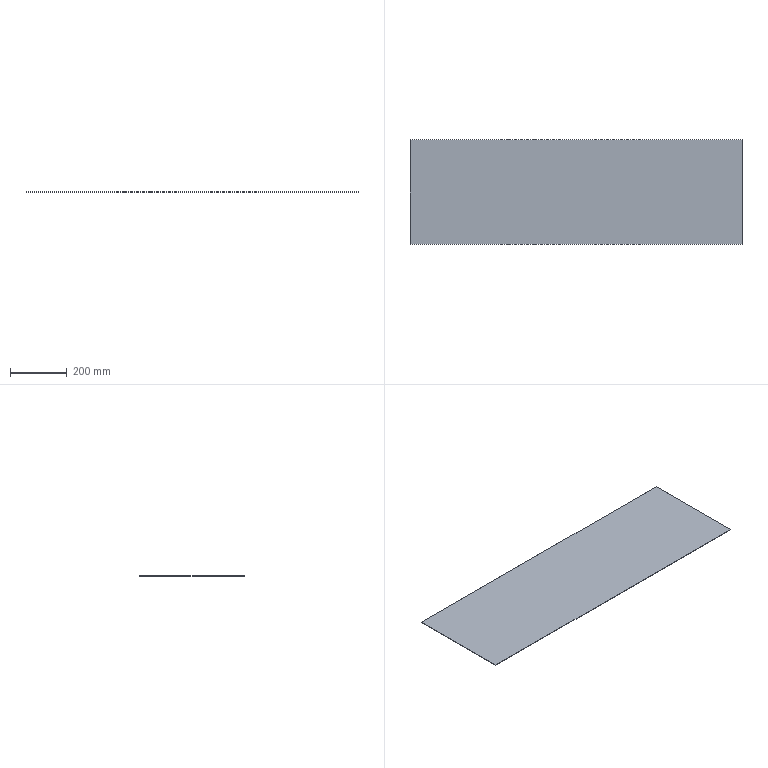Part | STEP file | JZBM | 1 solid | 6 faces | box 1170 x 370 x 1.5 mm | volume 649350 mm3 | plane 6
STEP:
#1=CARTESIAN_POINT('',(0.,0.,0.));
#2=DIRECTION('',(0.,0.,1.));
#3=DIRECTION('',(1.,0.,0.));
#4=AXIS2_PLACEMENT_3D('',#1,#2,#3);
#5=CARTESIAN_POINT('',(-585.,185.,0.));
#6=VERTEX_POINT('',#5);
#7=CARTESIAN_POINT('',(-585.,-185.,0.));
#8=VERTEX_POINT('',#7);
#9=CARTESIAN_POINT('',(-585.,185.,0.));
#10=DIRECTION('',(0.,-1.,0.));
#11=VECTOR('',#10,1.);
#12=LINE('',#9,#11);
#13=CARTESIAN_POINT('',(-585.,185.,1.5));
#14=DIRECTION('',(1.,0.,0.));
#15=DIRECTION('',(0.,0.,-1.));
#16=AXIS2_PLACEMENT_3D('',#13,#14,#15);
#17=PLANE('',#16);
#18=CARTESIAN_POINT('',(1.5,0.));
#19=DIRECTION('',(0.,-1.));
#20=VECTOR('',#19,1.);
#21=LINE('',#18,#20);
#22=(GEOMETRIC_REPRESENTATION_CONTEXT(2)PARAMETRIC_REPRESENTATION_CONTEXT()REPRESENTATION_CONTEXT('',''));
#23=DEFINITIONAL_REPRESENTATION('',(#21),#22);
#24=PCURVE('',#17,#23);
#25=CARTESIAN_POINT('',(-585.,-185.,0.));
#26=DIRECTION('',(0.,0.,1.));
#27=DIRECTION('',(1.,0.,0.));
#28=AXIS2_PLACEMENT_3D('',#25,#26,#27);
#29=PLANE('',#28);
#30=CARTESIAN_POINT('',(0.,370.));
#31=DIRECTION('',(0.,-1.));
#32=VECTOR('',#31,1.);
#33=LINE('',#30,#32);
#34=(GEOMETRIC_REPRESENTATION_CONTEXT(2)PARAMETRIC_REPRESENTATION_CONTEXT()REPRESENTATION_CONTEXT('',''));
#35=DEFINITIONAL_REPRESENTATION('',(#33),#34);
#36=PCURVE('',#29,#35);
#37=SURFACE_CURVE('',#12,(#24,#36),.PCURVE_S1.);
#38=EDGE_CURVE('',#6,#8,#37,.T.);
#39=ORIENTED_EDGE('',*,*,#38,.T.);
#40=CARTESIAN_POINT('',(-585.,-185.,1.5));
#41=VERTEX_POINT('',#40);
#42=CARTESIAN_POINT('',(-585.,-185.,1.5));
#43=DIRECTION('',(0.,0.,-1.));
#44=VECTOR('',#43,1.);
#45=LINE('',#42,#44);
#46=CARTESIAN_POINT('',(0.,-370.));
#47=DIRECTION('',(1.,0.));
#48=VECTOR('',#47,1.);
#49=LINE('',#46,#48);
#50=(GEOMETRIC_REPRESENTATION_CONTEXT(2)PARAMETRIC_REPRESENTATION_CONTEXT()REPRESENTATION_CONTEXT('',''));
#51=DEFINITIONAL_REPRESENTATION('',(#49),#50);
#52=PCURVE('',#17,#51);
#53=CARTESIAN_POINT('',(-585.,-185.,1.5));
#54=DIRECTION('',(0.,1.,0.));
#55=DIRECTION('',(0.,0.,1.));
#56=AXIS2_PLACEMENT_3D('',#53,#54,#55);
#57=PLANE('',#56);
#58=CARTESIAN_POINT('',(0.,0.));
#59=DIRECTION('',(-1.,0.));
#60=VECTOR('',#59,1.);
#61=LINE('',#58,#60);
#62=(GEOMETRIC_REPRESENTATION_CONTEXT(2)PARAMETRIC_REPRESENTATION_CONTEXT()REPRESENTATION_CONTEXT('',''));
#63=DEFINITIONAL_REPRESENTATION('',(#61),#62);
#64=PCURVE('',#57,#63);
#65=SURFACE_CURVE('',#45,(#52,#64),.PCURVE_S1.);
#66=EDGE_CURVE('',#41,#8,#65,.T.);
#67=ORIENTED_EDGE('',*,*,#66,.F.);
#68=CARTESIAN_POINT('',(-585.,185.,1.5));
#69=VERTEX_POINT('',#68);
#70=CARTESIAN_POINT('',(-585.,185.,1.5));
#71=DIRECTION('',(0.,-1.,0.));
#72=VECTOR('',#71,1.);
#73=LINE('',#70,#72);
#74=CARTESIAN_POINT('',(0.,0.));
#75=DIRECTION('',(0.,-1.));
#76=VECTOR('',#75,1.);
#77=LINE('',#74,#76);
#78=(GEOMETRIC_REPRESENTATION_CONTEXT(2)PARAMETRIC_REPRESENTATION_CONTEXT()REPRESENTATION_CONTEXT('',''));
#79=DEFINITIONAL_REPRESENTATION('',(#77),#78);
#80=PCURVE('',#17,#79);
#81=CARTESIAN_POINT('',(-585.,-185.,1.5));
#82=DIRECTION('',(0.,0.,1.));
#83=DIRECTION('',(1.,0.,0.));
#84=AXIS2_PLACEMENT_3D('',#81,#82,#83);
#85=PLANE('',#84);
#86=CARTESIAN_POINT('',(0.,370.));
#87=DIRECTION('',(0.,-1.));
#88=VECTOR('',#87,1.);
#89=LINE('',#86,#88);
#90=(GEOMETRIC_REPRESENTATION_CONTEXT(2)PARAMETRIC_REPRESENTATION_CONTEXT()REPRESENTATION_CONTEXT('',''));
#91=DEFINITIONAL_REPRESENTATION('',(#89),#90);
#92=PCURVE('',#85,#91);
#93=SURFACE_CURVE('',#73,(#80,#92),.PCURVE_S1.);
#94=EDGE_CURVE('',#69,#41,#93,.T.);
#95=ORIENTED_EDGE('',*,*,#94,.F.);
#96=CARTESIAN_POINT('',(-585.,185.,1.5));
#97=DIRECTION('',(0.,0.,-1.));
#98=VECTOR('',#97,1.);
#99=LINE('',#96,#98);
#100=CARTESIAN_POINT('',(0.,0.));
#101=DIRECTION('',(1.,0.));
#102=VECTOR('',#101,1.);
#103=LINE('',#100,#102);
#104=(GEOMETRIC_REPRESENTATION_CONTEXT(2)PARAMETRIC_REPRESENTATION_CONTEXT()REPRESENTATION_CONTEXT('',''));
#105=DEFINITIONAL_REPRESENTATION('',(#103),#104);
#106=PCURVE('',#17,#105);
#107=CARTESIAN_POINT('',(-585.,185.,1.5));
#108=DIRECTION('',(0.,-1.,0.));
#109=DIRECTION('',(0.,0.,-1.));
#110=AXIS2_PLACEMENT_3D('',#107,#108,#109);
#111=PLANE('',#110);
#112=CARTESIAN_POINT('',(0.,0.));
#113=DIRECTION('',(1.,0.));
#114=VECTOR('',#113,1.);
#115=LINE('',#112,#114);
#116=(GEOMETRIC_REPRESENTATION_CONTEXT(2)PARAMETRIC_REPRESENTATION_CONTEXT()REPRESENTATION_CONTEXT('',''));
#117=DEFINITIONAL_REPRESENTATION('',(#115),#116);
#118=PCURVE('',#111,#117);
#119=SURFACE_CURVE('',#99,(#106,#118),.PCURVE_S1.);
#120=EDGE_CURVE('',#69,#6,#119,.T.);
#121=ORIENTED_EDGE('',*,*,#120,.T.);
#122=EDGE_LOOP('',(#39,#67,#95,#121));
#123=FACE_BOUND('',#122,.T.);
#124=ADVANCED_FACE('',(#123),#17,.F.);
#125=CARTESIAN_POINT('',(585.,-185.,0.));
#126=VERTEX_POINT('',#125);
#127=CARTESIAN_POINT('',(-585.,-185.,0.));
#128=DIRECTION('',(1.,0.,0.));
#129=VECTOR('',#128,1.);
#130=LINE('',#127,#129);
#131=CARTESIAN_POINT('',(-1.5,0.));
#132=DIRECTION('',(0.,1.));
#133=VECTOR('',#132,1.);
#134=LINE('',#131,#133);
#135=(GEOMETRIC_REPRESENTATION_CONTEXT(2)PARAMETRIC_REPRESENTATION_CONTEXT()REPRESENTATION_CONTEXT('',''));
#136=DEFINITIONAL_REPRESENTATION('',(#134),#135);
#137=PCURVE('',#57,#136);
#138=CARTESIAN_POINT('',(0.,0.));
#139=DIRECTION('',(1.,0.));
#140=VECTOR('',#139,1.);
#141=LINE('',#138,#140);
#142=(GEOMETRIC_REPRESENTATION_CONTEXT(2)PARAMETRIC_REPRESENTATION_CONTEXT()REPRESENTATION_CONTEXT('',''));
#143=DEFINITIONAL_REPRESENTATION('',(#141),#142);
#144=PCURVE('',#29,#143);
#145=SURFACE_CURVE('',#130,(#137,#144),.PCURVE_S1.);
#146=EDGE_CURVE('',#8,#126,#145,.T.);
#147=ORIENTED_EDGE('',*,*,#146,.T.);
#148=CARTESIAN_POINT('',(585.,-185.,1.5));
#149=VERTEX_POINT('',#148);
#150=CARTESIAN_POINT('',(585.,-185.,1.5));
#151=DIRECTION('',(0.,0.,-1.));
#152=VECTOR('',#151,1.);
#153=LINE('',#150,#152);
#154=CARTESIAN_POINT('',(0.,1170.));
#155=DIRECTION('',(-1.,0.));
#156=VECTOR('',#155,1.);
#157=LINE('',#154,#156);
#158=(GEOMETRIC_REPRESENTATION_CONTEXT(2)PARAMETRIC_REPRESENTATION_CONTEXT()REPRESENTATION_CONTEXT('',''));
#159=DEFINITIONAL_REPRESENTATION('',(#157),#158);
#160=PCURVE('',#57,#159);
#161=CARTESIAN_POINT('',(585.,185.,1.5));
#162=DIRECTION('',(-1.,0.,0.));
#163=DIRECTION('',(0.,0.,1.));
#164=AXIS2_PLACEMENT_3D('',#161,#162,#163);
#165=PLANE('',#164);
#166=CARTESIAN_POINT('',(0.,-370.));
#167=DIRECTION('',(-1.,0.));
#168=VECTOR('',#167,1.);
#169=LINE('',#166,#168);
#170=(GEOMETRIC_REPRESENTATION_CONTEXT(2)PARAMETRIC_REPRESENTATION_CONTEXT()REPRESENTATION_CONTEXT('',''));
#171=DEFINITIONAL_REPRESENTATION('',(#169),#170);
#172=PCURVE('',#165,#171);
#173=SURFACE_CURVE('',#153,(#160,#172),.PCURVE_S1.);
#174=EDGE_CURVE('',#149,#126,#173,.T.);
#175=ORIENTED_EDGE('',*,*,#174,.F.);
#176=CARTESIAN_POINT('',(-585.,-185.,1.5));
#177=DIRECTION('',(1.,0.,0.));
#178=VECTOR('',#177,1.);
#179=LINE('',#176,#178);
#180=CARTESIAN_POINT('',(0.,0.));
#181=DIRECTION('',(0.,1.));
#182=VECTOR('',#181,1.);
#183=LINE('',#180,#182);
#184=(GEOMETRIC_REPRESENTATION_CONTEXT(2)PARAMETRIC_REPRESENTATION_CONTEXT()REPRESENTATION_CONTEXT('',''));
#185=DEFINITIONAL_REPRESENTATION('',(#183),#184);
#186=PCURVE('',#57,#185);
#187=CARTESIAN_POINT('',(0.,0.));
#188=DIRECTION('',(1.,0.));
#189=VECTOR('',#188,1.);
#190=LINE('',#187,#189);
#191=(GEOMETRIC_REPRESENTATION_CONTEXT(2)PARAMETRIC_REPRESENTATION_CONTEXT()REPRESENTATION_CONTEXT('',''));
#192=DEFINITIONAL_REPRESENTATION('',(#190),#191);
#193=PCURVE('',#85,#192);
#194=SURFACE_CURVE('',#179,(#186,#193),.PCURVE_S1.);
#195=EDGE_CURVE('',#41,#149,#194,.T.);
#196=ORIENTED_EDGE('',*,*,#195,.F.);
#197=ORIENTED_EDGE('',*,*,#66,.T.);
#198=EDGE_LOOP('',(#147,#175,#196,#197));
#199=FACE_BOUND('',#198,.T.);
#200=ADVANCED_FACE('',(#199),#57,.F.);
#201=CARTESIAN_POINT('',(585.,185.,0.));
#202=VERTEX_POINT('',#201);
#203=CARTESIAN_POINT('',(585.,185.,0.));
#204=DIRECTION('',(0.,1.,0.));
#205=VECTOR('',#204,1.);
#206=LINE('',#203,#205);
#207=CARTESIAN_POINT('',(-1.5,0.));
#208=DIRECTION('',(0.,1.));
#209=VECTOR('',#208,1.);
#210=LINE('',#207,#209);
#211=(GEOMETRIC_REPRESENTATION_CONTEXT(2)PARAMETRIC_REPRESENTATION_CONTEXT()REPRESENTATION_CONTEXT('',''));
#212=DEFINITIONAL_REPRESENTATION('',(#210),#211);
#213=PCURVE('',#165,#212);
#214=CARTESIAN_POINT('',(1170.,370.));
#215=DIRECTION('',(0.,1.));
#216=VECTOR('',#215,1.);
#217=LINE('',#214,#216);
#218=(GEOMETRIC_REPRESENTATION_CONTEXT(2)PARAMETRIC_REPRESENTATION_CONTEXT()REPRESENTATION_CONTEXT('',''));
#219=DEFINITIONAL_REPRESENTATION('',(#217),#218);
#220=PCURVE('',#29,#219);
#221=SURFACE_CURVE('',#206,(#213,#220),.PCURVE_S1.);
#222=EDGE_CURVE('',#126,#202,#221,.T.);
#223=ORIENTED_EDGE('',*,*,#222,.T.);
#224=CARTESIAN_POINT('',(585.,185.,1.5));
#225=VERTEX_POINT('',#224);
#226=CARTESIAN_POINT('',(585.,185.,1.5));
#227=DIRECTION('',(0.,0.,-1.));
#228=VECTOR('',#227,1.);
#229=LINE('',#226,#228);
#230=CARTESIAN_POINT('',(0.,0.));
#231=DIRECTION('',(-1.,0.));
#232=VECTOR('',#231,1.);
#233=LINE('',#230,#232);
#234=(GEOMETRIC_REPRESENTATION_CONTEXT(2)PARAMETRIC_REPRESENTATION_CONTEXT()REPRESENTATION_CONTEXT('',''));
#235=DEFINITIONAL_REPRESENTATION('',(#233),#234);
#236=PCURVE('',#165,#235);
#237=CARTESIAN_POINT('',(0.,1170.));
#238=DIRECTION('',(1.,0.));
#239=VECTOR('',#238,1.);
#240=LINE('',#237,#239);
#241=(GEOMETRIC_REPRESENTATION_CONTEXT(2)PARAMETRIC_REPRESENTATION_CONTEXT()REPRESENTATION_CONTEXT('',''));
#242=DEFINITIONAL_REPRESENTATION('',(#240),#241);
#243=PCURVE('',#111,#242);
#244=SURFACE_CURVE('',#229,(#236,#243),.PCURVE_S1.);
#245=EDGE_CURVE('',#225,#202,#244,.T.);
#246=ORIENTED_EDGE('',*,*,#245,.F.);
#247=CARTESIAN_POINT('',(585.,185.,1.5));
#248=DIRECTION('',(0.,1.,0.));
#249=VECTOR('',#248,1.);
#250=LINE('',#247,#249);
#251=CARTESIAN_POINT('',(0.,0.));
#252=DIRECTION('',(0.,1.));
#253=VECTOR('',#252,1.);
#254=LINE('',#251,#253);
#255=(GEOMETRIC_REPRESENTATION_CONTEXT(2)PARAMETRIC_REPRESENTATION_CONTEXT()REPRESENTATION_CONTEXT('',''));
#256=DEFINITIONAL_REPRESENTATION('',(#254),#255);
#257=PCURVE('',#165,#256);
#258=CARTESIAN_POINT('',(1170.,370.));
#259=DIRECTION('',(0.,1.));
#260=VECTOR('',#259,1.);
#261=LINE('',#258,#260);
#262=(GEOMETRIC_REPRESENTATION_CONTEXT(2)PARAMETRIC_REPRESENTATION_CONTEXT()REPRESENTATION_CONTEXT('',''));
#263=DEFINITIONAL_REPRESENTATION('',(#261),#262);
#264=PCURVE('',#85,#263);
#265=SURFACE_CURVE('',#250,(#257,#264),.PCURVE_S1.);
#266=EDGE_CURVE('',#149,#225,#265,.T.);
#267=ORIENTED_EDGE('',*,*,#266,.F.);
#268=ORIENTED_EDGE('',*,*,#174,.T.);
#269=EDGE_LOOP('',(#223,#246,#267,#268));
#270=FACE_BOUND('',#269,.T.);
#271=ADVANCED_FACE('',(#270),#165,.F.);
#272=CARTESIAN_POINT('',(-585.,185.,0.));
#273=DIRECTION('',(-1.,0.,0.));
#274=VECTOR('',#273,1.);
#275=LINE('',#272,#274);
#276=CARTESIAN_POINT('',(1.5,0.));
#277=DIRECTION('',(0.,-1.));
#278=VECTOR('',#277,1.);
#279=LINE('',#276,#278);
#280=(GEOMETRIC_REPRESENTATION_CONTEXT(2)PARAMETRIC_REPRESENTATION_CONTEXT()REPRESENTATION_CONTEXT('',''));
#281=DEFINITIONAL_REPRESENTATION('',(#279),#280);
#282=PCURVE('',#111,#281);
#283=CARTESIAN_POINT('',(0.,370.));
#284=DIRECTION('',(-1.,0.));
#285=VECTOR('',#284,1.);
#286=LINE('',#283,#285);
#287=(GEOMETRIC_REPRESENTATION_CONTEXT(2)PARAMETRIC_REPRESENTATION_CONTEXT()REPRESENTATION_CONTEXT('',''));
#288=DEFINITIONAL_REPRESENTATION('',(#286),#287);
#289=PCURVE('',#29,#288);
#290=SURFACE_CURVE('',#275,(#282,#289),.PCURVE_S1.);
#291=EDGE_CURVE('',#202,#6,#290,.T.);
#292=ORIENTED_EDGE('',*,*,#291,.T.);
#293=ORIENTED_EDGE('',*,*,#120,.F.);
#294=CARTESIAN_POINT('',(-585.,185.,1.5));
#295=DIRECTION('',(-1.,0.,0.));
#296=VECTOR('',#295,1.);
#297=LINE('',#294,#296);
#298=CARTESIAN_POINT('',(0.,0.));
#299=DIRECTION('',(0.,-1.));
#300=VECTOR('',#299,1.);
#301=LINE('',#298,#300);
#302=(GEOMETRIC_REPRESENTATION_CONTEXT(2)PARAMETRIC_REPRESENTATION_CONTEXT()REPRESENTATION_CONTEXT('',''));
#303=DEFINITIONAL_REPRESENTATION('',(#301),#302);
#304=PCURVE('',#111,#303);
#305=CARTESIAN_POINT('',(0.,370.));
#306=DIRECTION('',(-1.,0.));
#307=VECTOR('',#306,1.);
#308=LINE('',#305,#307);
#309=(GEOMETRIC_REPRESENTATION_CONTEXT(2)PARAMETRIC_REPRESENTATION_CONTEXT()REPRESENTATION_CONTEXT('',''));
#310=DEFINITIONAL_REPRESENTATION('',(#308),#309);
#311=PCURVE('',#85,#310);
#312=SURFACE_CURVE('',#297,(#304,#311),.PCURVE_S1.);
#313=EDGE_CURVE('',#225,#69,#312,.T.);
#314=ORIENTED_EDGE('',*,*,#313,.F.);
#315=ORIENTED_EDGE('',*,*,#245,.T.);
#316=EDGE_LOOP('',(#292,#293,#314,#315));
#317=FACE_BOUND('',#316,.T.);
#318=ADVANCED_FACE('',(#317),#111,.F.);
#319=ORIENTED_EDGE('',*,*,#94,.T.);
#320=ORIENTED_EDGE('',*,*,#195,.T.);
#321=ORIENTED_EDGE('',*,*,#266,.T.);
#322=ORIENTED_EDGE('',*,*,#313,.T.);
#323=EDGE_LOOP('',(#319,#320,#321,#322));
#324=FACE_BOUND('',#323,.T.);
#325=ADVANCED_FACE('',(#324),#85,.T.);
#326=ORIENTED_EDGE('',*,*,#38,.F.);
#327=ORIENTED_EDGE('',*,*,#291,.F.);
#328=ORIENTED_EDGE('',*,*,#222,.F.);
#329=ORIENTED_EDGE('',*,*,#146,.F.);
#330=EDGE_LOOP('',(#326,#327,#328,#329));
#331=FACE_BOUND('',#330,.T.);
#332=ADVANCED_FACE('',(#331),#29,.F.);
#333=CLOSED_SHELL('',(#124,#200,#271,#318,#325,#332));
#334=MANIFOLD_SOLID_BREP('',#333);
#335=(LENGTH_UNIT()NAMED_UNIT(*)SI_UNIT(.MILLI.,.METRE.));
#336=UNCERTAINTY_MEASURE_WITH_UNIT(LENGTH_MEASURE(0.0000001),#335,'','');
#337=(NAMED_UNIT(*)PLANE_ANGLE_UNIT()SI_UNIT($,.RADIAN.));
#338=(NAMED_UNIT(*)SI_UNIT($,.STERADIAN.)SOLID_ANGLE_UNIT());
#339=(GEOMETRIC_REPRESENTATION_CONTEXT(3)GLOBAL_UNCERTAINTY_ASSIGNED_CONTEXT((#336))GLOBAL_UNIT_ASSIGNED_CONTEXT((#335,#337,#338))REPRESENTATION_CONTEXT('',''));
#340=ADVANCED_BREP_SHAPE_REPRESENTATION('',(#4,#334),#339);